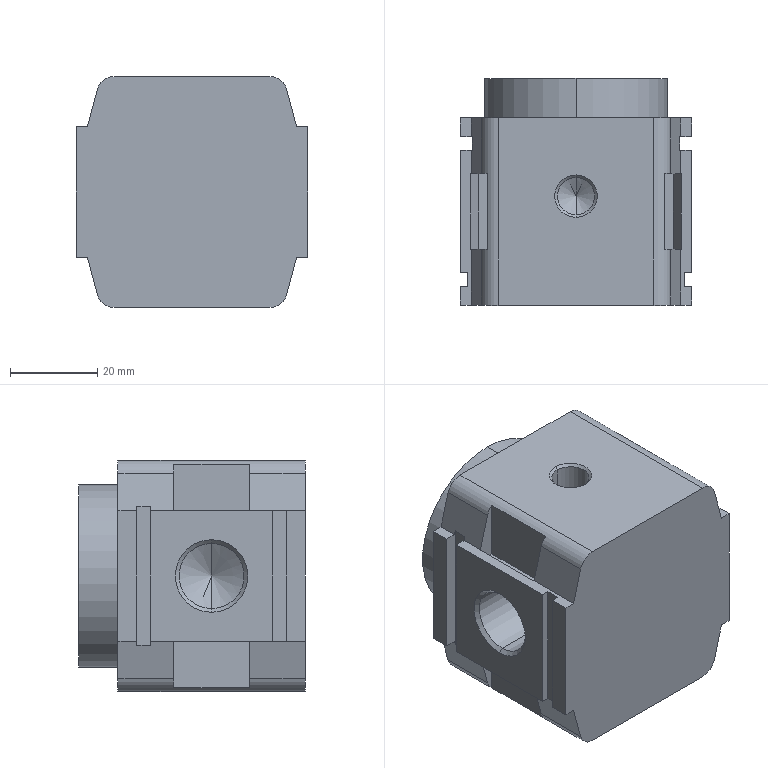Part | SolidWorks | features BaseBody 1 | 1 solid | 139 faces | box 53 x 52 x 53 mm | volume 114626 mm3 | plane 99 | cylinder 24 | cone 16 | commonest cylinder face diameters 8 x4 8.566 x4 14.95 x4 36.4 x2 42 x2 0.742 x1